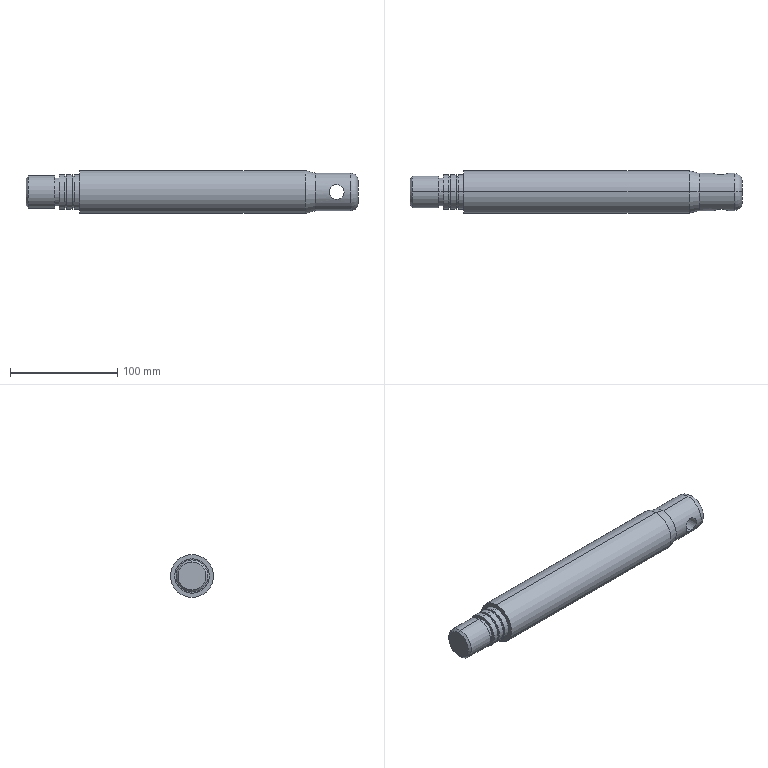Part | SolidWorks | features Chamfer 1, Fillet 1, ICE 1, Revolution 1 | 1 solid | 35 faces | box 310 x 40 x 40 mm | volume 342944 mm3 | cylinder 20 | plane 9 | cone 4 | torus 2 | commonest cylinder face diameters 32 x6 29 x4 14 x2 26 x2 30 x2 35 x2
STEP:
#1=CARTESIAN_POINT('',(310.,0.,-10.5));
#2=VERTEX_POINT('',#1);
#3=CARTESIAN_POINT('',(310.,0.,10.5));
#4=VERTEX_POINT('',#3);
#5=CARTESIAN_POINT('',(310.,0.,0.));
#6=DIRECTION('',(1.,0.,0.));
#7=DIRECTION('',(0.,0.,1.));
#8=AXIS2_PLACEMENT_3D('',#5,#6,#7);
#9=CIRCLE('',#8,10.5);
#10=EDGE_CURVE('',#2,#4,#9,.T.);
#11=ORIENTED_EDGE('',*,*,#10,.F.);
#12=CARTESIAN_POINT('',(303.,0.,-17.5));
#13=VERTEX_POINT('',#12);
#14=CARTESIAN_POINT('',(303.,0.,-10.5));
#15=DIRECTION('',(0.,1.,0.));
#16=DIRECTION('',(0.,0.,1.));
#17=AXIS2_PLACEMENT_3D('',#14,#15,#16);
#18=CIRCLE('',#17,7.);
#19=EDGE_CURVE('',#2,#13,#18,.T.);
#20=ORIENTED_EDGE('',*,*,#19,.T.);
#21=CARTESIAN_POINT('',(303.,0.,17.5));
#22=VERTEX_POINT('',#21);
#23=CARTESIAN_POINT('',(303.,0.,0.));
#24=DIRECTION('',(-1.,0.,0.));
#25=DIRECTION('',(0.,0.,1.));
#26=AXIS2_PLACEMENT_3D('',#23,#24,#25);
#27=CIRCLE('',#26,17.5);
#28=EDGE_CURVE('',#22,#13,#27,.T.);
#29=ORIENTED_EDGE('',*,*,#28,.F.);
#30=CARTESIAN_POINT('',(303.,0.,10.5));
#31=DIRECTION('',(0.,-1.,0.));
#32=DIRECTION('',(0.,0.,-1.));
#33=AXIS2_PLACEMENT_3D('',#30,#31,#32);
#34=CIRCLE('',#33,7.);
#35=EDGE_CURVE('',#4,#22,#34,.T.);
#36=ORIENTED_EDGE('',*,*,#35,.F.);
#37=EDGE_LOOP('',(#11,#20,#29,#36));
#38=FACE_OUTER_BOUND('',#37,.T.);
#39=CARTESIAN_POINT('',(303.,0.,0.));
#40=DIRECTION('',(-1.,0.,0.));
#41=DIRECTION('',(0.,0.,1.));
#42=AXIS2_PLACEMENT_3D('',#39,#40,#41);
#43=TOROIDAL_SURFACE('',#42,10.5,7.);
#44=ADVANCED_FACE('',(#38),#43,.T.);
#45=CARTESIAN_POINT('',(0.,0.,13.));
#46=VERTEX_POINT('',#45);
#47=CARTESIAN_POINT('',(0.,0.,-13.));
#48=VERTEX_POINT('',#47);
#49=CARTESIAN_POINT('',(0.,0.,0.));
#50=DIRECTION('',(-1.,0.,0.));
#51=DIRECTION('',(0.,0.,-1.));
#52=AXIS2_PLACEMENT_3D('',#49,#50,#51);
#53=CIRCLE('',#52,13.);
#54=EDGE_CURVE('',#46,#48,#53,.T.);
#55=ORIENTED_EDGE('',*,*,#54,.F.);
#56=CARTESIAN_POINT('',(2.,0.,15.));
#57=VERTEX_POINT('',#56);
#58=CARTESIAN_POINT('',(0.,0.,13.));
#59=DIRECTION('',(0.7071,0.,0.7071));
#60=VECTOR('',#59,1000.);
#61=LINE('',#58,#60);
#62=EDGE_CURVE('',#46,#57,#61,.T.);
#63=ORIENTED_EDGE('',*,*,#62,.T.);
#64=CARTESIAN_POINT('',(2.,0.,-15.));
#65=VERTEX_POINT('',#64);
#66=CARTESIAN_POINT('',(2.,0.,0.));
#67=DIRECTION('',(1.,0.,0.));
#68=DIRECTION('',(0.,0.,-1.));
#69=AXIS2_PLACEMENT_3D('',#66,#67,#68);
#70=CIRCLE('',#69,15.);
#71=EDGE_CURVE('',#65,#57,#70,.T.);
#72=ORIENTED_EDGE('',*,*,#71,.F.);
#73=CARTESIAN_POINT('',(0.,0.,-13.));
#74=DIRECTION('',(0.7071,0.,-0.7071));
#75=VECTOR('',#74,1000.);
#76=LINE('',#73,#75);
#77=EDGE_CURVE('',#48,#65,#76,.T.);
#78=ORIENTED_EDGE('',*,*,#77,.F.);
#79=EDGE_LOOP('',(#55,#63,#72,#78));
#80=FACE_OUTER_BOUND('',#79,.T.);
#81=CARTESIAN_POINT('',(0.,0.,0.));
#82=DIRECTION('',(1.,0.,0.));
#83=DIRECTION('',(0.,0.,-1.));
#84=AXIS2_PLACEMENT_3D('',#81,#82,#83);
#85=CONICAL_SURFACE('',#84,13.,0.7854);
#86=ADVANCED_FACE('',(#80),#85,.T.);
#87=CARTESIAN_POINT('',(290.,-16.039,-7.));
#88=VERTEX_POINT('',#87);
#89=CARTESIAN_POINT('',(290.,-16.039,7.));
#90=VERTEX_POINT('',#89);
#91=CARTESIAN_POINT('',(290.,-16.039,-7.));
#92=CARTESIAN_POINT('',(289.77,-16.039,-7.));
#93=CARTESIAN_POINT('',(289.54,-16.044,-6.989));
#94=CARTESIAN_POINT('',(289.079,-16.064,-6.943));
#95=CARTESIAN_POINT('',(288.847,-16.079,-6.908));
#96=CARTESIAN_POINT('',(288.167,-16.137,-6.771));
#97=CARTESIAN_POINT('',(287.729,-16.194,-6.637));
#98=CARTESIAN_POINT('',(287.095,-16.299,-6.373));
#99=CARTESIAN_POINT('',(286.886,-16.337,-6.273));
#100=CARTESIAN_POINT('',(286.483,-16.419,-6.057));
#101=CARTESIAN_POINT('',(286.288,-16.462,-5.939));
#102=CARTESIAN_POINT('',(285.724,-16.595,-5.561));
#103=CARTESIAN_POINT('',(285.373,-16.69,-5.272));
#104=CARTESIAN_POINT('',(284.728,-16.881,-4.627));
#105=CARTESIAN_POINT('',(284.441,-16.973,-4.278));
#106=CARTESIAN_POINT('',(284.062,-17.102,-3.714));
#107=CARTESIAN_POINT('',(283.945,-17.144,-3.519));
#108=CARTESIAN_POINT('',(283.728,-17.222,-3.116));
#109=CARTESIAN_POINT('',(283.628,-17.258,-2.907));
#110=CARTESIAN_POINT('',(283.363,-17.357,-2.273));
#111=CARTESIAN_POINT('',(283.229,-17.409,-1.836));
#112=CARTESIAN_POINT('',(283.047,-17.481,-0.9335));
#113=CARTESIAN_POINT('',(283.,-17.5,-0.4644));
#114=CARTESIAN_POINT('',(283.,-17.5,0.4581));
#115=CARTESIAN_POINT('',(283.045,-17.482,0.9167));
#116=CARTESIAN_POINT('',(283.227,-17.41,1.829));
#117=CARTESIAN_POINT('',(283.363,-17.357,2.27));
#118=CARTESIAN_POINT('',(283.626,-17.259,2.903));
#119=CARTESIAN_POINT('',(283.724,-17.223,3.109));
#120=CARTESIAN_POINT('',(283.941,-17.145,3.513));
#121=CARTESIAN_POINT('',(284.06,-17.103,3.711));
#122=CARTESIAN_POINT('',(284.44,-16.974,4.278));
#123=CARTESIAN_POINT('',(284.727,-16.881,4.627));
#124=CARTESIAN_POINT('',(285.209,-16.739,5.108));
#125=CARTESIAN_POINT('',(285.378,-16.691,5.262));
#126=CARTESIAN_POINT('',(285.73,-16.597,5.551));
#127=CARTESIAN_POINT('',(285.912,-16.551,5.687));
#128=CARTESIAN_POINT('',(286.475,-16.418,6.064));
#129=CARTESIAN_POINT('',(286.874,-16.335,6.28));
#130=CARTESIAN_POINT('',(287.725,-16.194,6.636));
#131=CARTESIAN_POINT('',(288.165,-16.137,6.771));
#132=CARTESIAN_POINT('',(288.841,-16.079,6.907));
#133=CARTESIAN_POINT('',(289.069,-16.064,6.942));
#134=CARTESIAN_POINT('',(289.532,-16.044,6.988));
#135=CARTESIAN_POINT('',(289.766,-16.039,7.));
#136=CARTESIAN_POINT('',(290.,-16.039,7.));
#137=B_SPLINE_CURVE_WITH_KNOTS('',3,(#91,#92,#93,#94,#95,#96,#97,#98,#99,#100,#101,#102,#103,#104,#105,#106,#107,#108,#109,#110,#111,#112,#113,#114,#115,#116,#117,#118,#119,#120,#121,#122,#123,#124,#125,#126,#127,#128,#129,#130,#131,#132,#133,#134,#135,#136),.UNSPECIFIED.,.F.,.F.,(4,2,2,2,2,2,2,2,2,2,2,2,2,2,2,2,2,2,2,2,2,2,4),(0.02212,0.02281,0.0235,0.02488,0.02557,0.02626,0.02764,0.02902,0.02971,0.0304,0.03179,0.03317,0.03455,0.03593,0.03662,0.03731,0.03869,0.03938,0.04007,0.04145,0.04283,0.04353,0.04422),.UNSPECIFIED.);
#138=EDGE_CURVE('',#88,#90,#137,.T.);
#139=ORIENTED_EDGE('',*,*,#138,.F.);
#140=CARTESIAN_POINT('',(290.,16.039,-7.));
#141=VERTEX_POINT('',#140);
#142=CARTESIAN_POINT('',(290.,-20.,-7.));
#143=DIRECTION('',(0.,1.,0.));
#144=VECTOR('',#143,1000.);
#145=LINE('',#142,#144);
#146=EDGE_CURVE('',#88,#141,#145,.T.);
#147=ORIENTED_EDGE('',*,*,#146,.T.);
#148=CARTESIAN_POINT('',(290.,16.039,7.));
#149=VERTEX_POINT('',#148);
#150=CARTESIAN_POINT('',(290.,16.039,7.));
#151=CARTESIAN_POINT('',(289.532,16.039,7.));
#152=CARTESIAN_POINT('',(289.073,16.059,6.954));
#153=CARTESIAN_POINT('',(288.397,16.117,6.818));
#154=CARTESIAN_POINT('',(288.174,16.141,6.762));
#155=CARTESIAN_POINT('',(287.732,16.197,6.626));
#156=CARTESIAN_POINT('',(287.514,16.229,6.548));
#157=CARTESIAN_POINT('',(286.88,16.334,6.283));
#158=CARTESIAN_POINT('',(286.48,16.417,6.068));
#159=CARTESIAN_POINT('',(285.912,16.551,5.687));
#160=CARTESIAN_POINT('',(285.728,16.597,5.55));
#161=CARTESIAN_POINT('',(285.377,16.691,5.261));
#162=CARTESIAN_POINT('',(285.21,16.738,5.109));
#163=CARTESIAN_POINT('',(284.731,16.88,4.63));
#164=CARTESIAN_POINT('',(284.441,16.973,4.279));
#165=CARTESIAN_POINT('',(283.931,17.147,3.518));
#166=CARTESIAN_POINT('',(283.716,17.225,3.118));
#167=CARTESIAN_POINT('',(283.453,17.324,2.487));
#168=CARTESIAN_POINT('',(283.375,17.353,2.271));
#169=CARTESIAN_POINT('',(283.24,17.405,1.83));
#170=CARTESIAN_POINT('',(283.182,17.428,1.603));
#171=CARTESIAN_POINT('',(283.046,17.482,0.9238));
#172=CARTESIAN_POINT('',(283.,17.5,0.466));
#173=CARTESIAN_POINT('',(283.,17.5,-0.2276));
#174=CARTESIAN_POINT('',(283.011,17.495,-0.4612));
#175=CARTESIAN_POINT('',(283.057,17.477,-0.9248));
#176=CARTESIAN_POINT('',(283.092,17.463,-1.153));
#177=CARTESIAN_POINT('',(283.228,17.41,-1.83));
#178=CARTESIAN_POINT('',(283.362,17.358,-2.27));
#179=CARTESIAN_POINT('',(283.719,17.224,-3.124));
#180=CARTESIAN_POINT('',(283.935,17.146,-3.525));
#181=CARTESIAN_POINT('',(284.441,16.973,-4.279));
#182=CARTESIAN_POINT('',(284.734,16.878,-4.635));
#183=CARTESIAN_POINT('',(285.376,16.689,-5.275));
#184=CARTESIAN_POINT('',(285.725,16.595,-5.561));
#185=CARTESIAN_POINT('',(286.292,16.461,-5.941));
#186=CARTESIAN_POINT('',(286.489,16.418,-6.06));
#187=CARTESIAN_POINT('',(286.892,16.336,-6.276));
#188=CARTESIAN_POINT('',(287.098,16.298,-6.374));
#189=CARTESIAN_POINT('',(287.728,16.194,-6.637));
#190=CARTESIAN_POINT('',(288.166,16.137,-6.771));
#191=CARTESIAN_POINT('',(288.849,16.079,-6.909));
#192=CARTESIAN_POINT('',(289.08,16.064,-6.943));
#193=CARTESIAN_POINT('',(289.54,16.044,-6.989));
#194=CARTESIAN_POINT('',(289.77,16.039,-7.));
#195=CARTESIAN_POINT('',(290.,16.039,-7.));
#196=B_SPLINE_CURVE_WITH_KNOTS('',3,(#150,#151,#152,#153,#154,#155,#156,#157,#158,#159,#160,#161,#162,#163,#164,#165,#166,#167,#168,#169,#170,#171,#172,#173,#174,#175,#176,#177,#178,#179,#180,#181,#182,#183,#184,#185,#186,#187,#188,#189,#190,#191,#192,#193,#194,#195),.UNSPECIFIED.,.F.,.F.,(4,2,2,2,2,2,2,2,2,2,2,2,2,2,2,2,2,2,2,2,2,2,4),(0.,0.001382,0.002074,0.002765,0.004147,0.004838,0.00553,0.006912,0.008294,0.008985,0.009677,0.01106,0.01175,0.01244,0.01382,0.01521,0.01659,0.01797,0.01866,0.01935,0.02074,0.02143,0.02212),.UNSPECIFIED.);
#197=EDGE_CURVE('',#149,#141,#196,.T.);
#198=ORIENTED_EDGE('',*,*,#197,.F.);
#199=CARTESIAN_POINT('',(290.,-20.,7.));
#200=DIRECTION('',(0.,1.,0.));
#201=VECTOR('',#200,1000.);
#202=LINE('',#199,#201);
#203=EDGE_CURVE('',#90,#149,#202,.T.);
#204=ORIENTED_EDGE('',*,*,#203,.F.);
#205=EDGE_LOOP('',(#139,#147,#198,#204));
#206=FACE_OUTER_BOUND('',#205,.T.);
#207=CARTESIAN_POINT('',(290.,-20.,0.));
#208=DIRECTION('',(0.,1.,0.));
#209=DIRECTION('',(0.,0.,1.));
#210=AXIS2_PLACEMENT_3D('',#207,#208,#209);
#211=CYLINDRICAL_SURFACE('',#210,7.);
#212=ADVANCED_FACE('',(#206),#211,.F.);
#213=ORIENTED_EDGE('',*,*,#197,.T.);
#214=CARTESIAN_POINT('',(290.,16.039,-7.));
#215=CARTESIAN_POINT('',(290.23,16.039,-7.));
#216=CARTESIAN_POINT('',(290.46,16.044,-6.989));
#217=CARTESIAN_POINT('',(290.921,16.064,-6.943));
#218=CARTESIAN_POINT('',(291.153,16.079,-6.908));
#219=CARTESIAN_POINT('',(291.833,16.137,-6.771));
#220=CARTESIAN_POINT('',(292.271,16.194,-6.637));
#221=CARTESIAN_POINT('',(292.905,16.299,-6.373));
#222=CARTESIAN_POINT('',(293.114,16.337,-6.273));
#223=CARTESIAN_POINT('',(293.517,16.419,-6.057));
#224=CARTESIAN_POINT('',(293.712,16.462,-5.939));
#225=CARTESIAN_POINT('',(294.276,16.595,-5.561));
#226=CARTESIAN_POINT('',(294.627,16.69,-5.272));
#227=CARTESIAN_POINT('',(295.272,16.881,-4.627));
#228=CARTESIAN_POINT('',(295.559,16.973,-4.278));
#229=CARTESIAN_POINT('',(295.938,17.102,-3.714));
#230=CARTESIAN_POINT('',(296.055,17.144,-3.519));
#231=CARTESIAN_POINT('',(296.272,17.222,-3.116));
#232=CARTESIAN_POINT('',(296.372,17.258,-2.907));
#233=CARTESIAN_POINT('',(296.637,17.357,-2.273));
#234=CARTESIAN_POINT('',(296.771,17.409,-1.836));
#235=CARTESIAN_POINT('',(296.953,17.481,-0.9335));
#236=CARTESIAN_POINT('',(297.,17.5,-0.4644));
#237=CARTESIAN_POINT('',(297.,17.5,0.4581));
#238=CARTESIAN_POINT('',(296.955,17.482,0.9167));
#239=CARTESIAN_POINT('',(296.773,17.41,1.829));
#240=CARTESIAN_POINT('',(296.637,17.357,2.27));
#241=CARTESIAN_POINT('',(296.374,17.259,2.903));
#242=CARTESIAN_POINT('',(296.276,17.223,3.109));
#243=CARTESIAN_POINT('',(296.059,17.145,3.513));
#244=CARTESIAN_POINT('',(295.94,17.103,3.711));
#245=CARTESIAN_POINT('',(295.56,16.974,4.278));
#246=CARTESIAN_POINT('',(295.273,16.881,4.627));
#247=CARTESIAN_POINT('',(294.791,16.739,5.108));
#248=CARTESIAN_POINT('',(294.622,16.691,5.262));
#249=CARTESIAN_POINT('',(294.27,16.597,5.551));
#250=CARTESIAN_POINT('',(294.088,16.551,5.687));
#251=CARTESIAN_POINT('',(293.525,16.418,6.064));
#252=CARTESIAN_POINT('',(293.126,16.335,6.28));
#253=CARTESIAN_POINT('',(292.275,16.194,6.636));
#254=CARTESIAN_POINT('',(291.835,16.137,6.771));
#255=CARTESIAN_POINT('',(291.159,16.079,6.907));
#256=CARTESIAN_POINT('',(290.931,16.064,6.942));
#257=CARTESIAN_POINT('',(290.468,16.044,6.988));
#258=CARTESIAN_POINT('',(290.234,16.039,7.));
#259=CARTESIAN_POINT('',(290.,16.039,7.));
#260=B_SPLINE_CURVE_WITH_KNOTS('',3,(#214,#215,#216,#217,#218,#219,#220,#221,#222,#223,#224,#225,#226,#227,#228,#229,#230,#231,#232,#233,#234,#235,#236,#237,#238,#239,#240,#241,#242,#243,#244,#245,#246,#247,#248,#249,#250,#251,#252,#253,#254,#255,#256,#257,#258,#259),.UNSPECIFIED.,.F.,.F.,(4,2,2,2,2,2,2,2,2,2,2,2,2,2,2,2,2,2,2,2,2,2,4),(0.02212,0.02281,0.0235,0.02488,0.02557,0.02626,0.02764,0.02902,0.02971,0.0304,0.03179,0.03317,0.03455,0.03593,0.03662,0.03731,0.03869,0.03938,0.04007,0.04145,0.04283,0.04353,0.04422),.UNSPECIFIED.);
#261=EDGE_CURVE('',#141,#149,#260,.T.);
#262=ORIENTED_EDGE('',*,*,#261,.T.);
#263=EDGE_LOOP('',(#213,#262));
#264=FACE_BOUND('',#263,.T.);
#265=ORIENTED_EDGE('',*,*,#28,.T.);
#266=CARTESIAN_POINT('',(270.,0.,-17.5));
#267=VERTEX_POINT('',#266);
#268=CARTESIAN_POINT('',(0.,0.,-17.5));
#269=DIRECTION('',(-1.,0.,0.));
#270=VECTOR('',#269,1000.);
#271=LINE('',#268,#270);
#272=EDGE_CURVE('',#13,#267,#271,.T.);
#273=ORIENTED_EDGE('',*,*,#272,.T.);
#274=CARTESIAN_POINT('',(270.,0.,17.5));
#275=VERTEX_POINT('',#274);
#276=CARTESIAN_POINT('',(270.,0.,0.));
#277=DIRECTION('',(-1.,0.,0.));
#278=DIRECTION('',(0.,0.,1.));
#279=AXIS2_PLACEMENT_3D('',#276,#277,#278);
#280=CIRCLE('',#279,17.5);
#281=EDGE_CURVE('',#275,#267,#280,.T.);
#282=ORIENTED_EDGE('',*,*,#281,.F.);
#283=CARTESIAN_POINT('',(0.,0.,17.5));
#284=DIRECTION('',(-1.,0.,0.));
#285=VECTOR('',#284,1000.);
#286=LINE('',#283,#285);
#287=EDGE_CURVE('',#22,#275,#286,.T.);
#288=ORIENTED_EDGE('',*,*,#287,.F.);
#289=EDGE_LOOP('',(#265,#273,#282,#288));
#290=FACE_OUTER_BOUND('',#289,.T.);
#291=CARTESIAN_POINT('',(0.,0.,0.));
#292=DIRECTION('',(-1.,0.,0.));
#293=DIRECTION('',(0.,0.,1.));
#294=AXIS2_PLACEMENT_3D('',#291,#292,#293);
#295=CYLINDRICAL_SURFACE('',#294,17.5);
#296=ADVANCED_FACE('',(#264,#290),#295,.T.);
#297=ORIENTED_EDGE('',*,*,#281,.T.);
#298=CARTESIAN_POINT('',(260.67,0.,-20.));
#299=VERTEX_POINT('',#298);
#300=CARTESIAN_POINT('',(270.,0.,-17.5));
#301=DIRECTION('',(-0.9659,0.,-0.2588));
#302=VECTOR('',#301,1000.);
#303=LINE('',#300,#302);
#304=EDGE_CURVE('',#267,#299,#303,.T.);
#305=ORIENTED_EDGE('',*,*,#304,.T.);
#306=CARTESIAN_POINT('',(260.67,0.,20.));
#307=VERTEX_POINT('',#306);
#308=CARTESIAN_POINT('',(260.67,0.,0.));
#309=DIRECTION('',(-1.,0.,0.));
#310=DIRECTION('',(0.,0.,1.));
#311=AXIS2_PLACEMENT_3D('',#308,#309,#310);
#312=CIRCLE('',#311,20.);
#313=EDGE_CURVE('',#307,#299,#312,.T.);
#314=ORIENTED_EDGE('',*,*,#313,.F.);
#315=CARTESIAN_POINT('',(270.,0.,17.5));
#316=DIRECTION('',(-0.9659,0.,0.2588));
#317=VECTOR('',#316,1000.);
#318=LINE('',#315,#317);
#319=EDGE_CURVE('',#275,#307,#318,.T.);
#320=ORIENTED_EDGE('',*,*,#319,.F.);
#321=EDGE_LOOP('',(#297,#305,#314,#320));
#322=FACE_OUTER_BOUND('',#321,.T.);
#323=CARTESIAN_POINT('',(270.,0.,0.));
#324=DIRECTION('',(-1.,0.,0.));
#325=DIRECTION('',(0.,0.,1.));
#326=AXIS2_PLACEMENT_3D('',#323,#324,#325);
#327=CONICAL_SURFACE('',#326,17.5,0.2618);
#328=ADVANCED_FACE('',(#322),#327,.T.);
#329=ORIENTED_EDGE('',*,*,#313,.T.);
#330=CARTESIAN_POINT('',(50.,0.,-20.));
#331=VERTEX_POINT('',#330);
#332=CARTESIAN_POINT('',(0.,0.,-20.));
#333=DIRECTION('',(-1.,0.,0.));
#334=VECTOR('',#333,1000.);
#335=LINE('',#332,#334);
#336=EDGE_CURVE('',#299,#331,#335,.T.);
#337=ORIENTED_EDGE('',*,*,#336,.T.);
#338=CARTESIAN_POINT('',(50.,0.,20.));
#339=VERTEX_POINT('',#338);
#340=CARTESIAN_POINT('',(50.,0.,0.));
#341=DIRECTION('',(-1.,0.,0.));
#342=DIRECTION('',(0.,0.,1.));
#343=AXIS2_PLACEMENT_3D('',#340,#341,#342);
#344=CIRCLE('',#343,20.);
#345=EDGE_CURVE('',#339,#331,#344,.T.);
#346=ORIENTED_EDGE('',*,*,#345,.F.);
#347=CARTESIAN_POINT('',(0.,0.,20.));
#348=DIRECTION('',(-1.,0.,0.));
#349=VECTOR('',#348,1000.);
#350=LINE('',#347,#349);
#351=EDGE_CURVE('',#307,#339,#350,.T.);
#352=ORIENTED_EDGE('',*,*,#351,.F.);
#353=EDGE_LOOP('',(#329,#337,#346,#352));
#354=FACE_OUTER_BOUND('',#353,.T.);
#355=CARTESIAN_POINT('',(0.,0.,0.));
#356=DIRECTION('',(-1.,0.,0.));
#357=DIRECTION('',(0.,0.,1.));
#358=AXIS2_PLACEMENT_3D('',#355,#356,#357);
#359=CYLINDRICAL_SURFACE('',#358,20.);
#360=ADVANCED_FACE('',(#354),#359,.T.);
#361=CARTESIAN_POINT('',(50.,0.,16.));
#362=VERTEX_POINT('',#361);
#363=CARTESIAN_POINT('',(50.,0.,-16.));
#364=VERTEX_POINT('',#363);
#365=CARTESIAN_POINT('',(50.,0.,0.));
#366=DIRECTION('',(-1.,0.,0.));
#367=DIRECTION('',(0.,0.,1.));
#368=AXIS2_PLACEMENT_3D('',#365,#366,#367);
#369=CIRCLE('',#368,16.);
#370=EDGE_CURVE('',#362,#364,#369,.T.);
#371=ORIENTED_EDGE('',*,*,#370,.T.);
#372=CARTESIAN_POINT('',(45.,0.,-16.));
#373=VERTEX_POINT('',#372);
#374=CARTESIAN_POINT('',(0.,0.,-16.));
#375=DIRECTION('',(-1.,0.,0.));
#376=VECTOR('',#375,1000.);
#377=LINE('',#374,#376);
#378=EDGE_CURVE('',#364,#373,#377,.T.);
#379=ORIENTED_EDGE('',*,*,#378,.T.);
#380=CARTESIAN_POINT('',(45.,0.,16.));
#381=VERTEX_POINT('',#380);
#382=CARTESIAN_POINT('',(45.,0.,0.));
#383=DIRECTION('',(-1.,0.,0.));
#384=DIRECTION('',(0.,0.,1.));
#385=AXIS2_PLACEMENT_3D('',#382,#383,#384);
#386=CIRCLE('',#385,16.);
#387=EDGE_CURVE('',#381,#373,#386,.T.);
#388=ORIENTED_EDGE('',*,*,#387,.F.);
#389=CARTESIAN_POINT('',(0.,0.,16.));
#390=DIRECTION('',(-1.,0.,0.));
#391=VECTOR('',#390,1000.);
#392=LINE('',#389,#391);
#393=EDGE_CURVE('',#362,#381,#392,.T.);
#394=ORIENTED_EDGE('',*,*,#393,.F.);
#395=EDGE_LOOP('',(#371,#379,#388,#394));
#396=FACE_OUTER_BOUND('',#395,.T.);
#397=CARTESIAN_POINT('',(0.,0.,0.));
#398=DIRECTION('',(-1.,0.,0.));
#399=DIRECTION('',(0.,0.,1.));
#400=AXIS2_PLACEMENT_3D('',#397,#398,#399);
#401=CYLINDRICAL_SURFACE('',#400,16.);
#402=ADVANCED_FACE('',(#396),#401,.T.);
#403=CARTESIAN_POINT('',(45.,0.,14.5));
#404=VERTEX_POINT('',#403);
#405=CARTESIAN_POINT('',(45.,0.,-14.5));
#406=VERTEX_POINT('',#405);
#407=CARTESIAN_POINT('',(45.,0.,0.));
#408=DIRECTION('',(-1.,0.,0.));
#409=DIRECTION('',(0.,0.,1.));
#410=AXIS2_PLACEMENT_3D('',#407,#408,#409);
#411=CIRCLE('',#410,14.5);
#412=EDGE_CURVE('',#404,#406,#411,.T.);
#413=ORIENTED_EDGE('',*,*,#412,.T.);
#414=CARTESIAN_POINT('',(43.,0.,-14.5));
#415=VERTEX_POINT('',#414);
#416=CARTESIAN_POINT('',(0.,0.,-14.5));
#417=DIRECTION('',(-1.,0.,0.));
#418=VECTOR('',#417,1000.);
#419=LINE('',#416,#418);
#420=EDGE_CURVE('',#406,#415,#419,.T.);
#421=ORIENTED_EDGE('',*,*,#420,.T.);
#422=CARTESIAN_POINT('',(43.,0.,14.5));
#423=VERTEX_POINT('',#422);
#424=CARTESIAN_POINT('',(43.,0.,0.));
#425=DIRECTION('',(-1.,0.,0.));
#426=DIRECTION('',(0.,0.,1.));
#427=AXIS2_PLACEMENT_3D('',#424,#425,#426);
#428=CIRCLE('',#427,14.5);
#429=EDGE_CURVE('',#423,#415,#428,.T.);
#430=ORIENTED_EDGE('',*,*,#429,.F.);
#431=CARTESIAN_POINT('',(0.,0.,14.5));
#432=DIRECTION('',(-1.,0.,0.));
#433=VECTOR('',#432,1000.);
#434=LINE('',#431,#433);
#435=EDGE_CURVE('',#404,#423,#434,.T.);
#436=ORIENTED_EDGE('',*,*,#435,.F.);
#437=EDGE_LOOP('',(#413,#421,#430,#436));
#438=FACE_OUTER_BOUND('',#437,.T.);
#439=CARTESIAN_POINT('',(0.,0.,0.));
#440=DIRECTION('',(-1.,0.,0.));
#441=DIRECTION('',(0.,0.,1.));
#442=AXIS2_PLACEMENT_3D('',#439,#440,#441);
#443=CYLINDRICAL_SURFACE('',#442,14.5);
#444=ADVANCED_FACE('',(#438),#443,.T.);
#445=CARTESIAN_POINT('',(43.,0.,16.));
#446=VERTEX_POINT('',#445);
#447=CARTESIAN_POINT('',(43.,0.,-16.));
#448=VERTEX_POINT('',#447);
#449=CARTESIAN_POINT('',(43.,0.,0.));
#450=DIRECTION('',(-1.,0.,0.));
#451=DIRECTION('',(0.,0.,1.));
#452=AXIS2_PLACEMENT_3D('',#449,#450,#451);
#453=CIRCLE('',#452,16.);
#454=EDGE_CURVE('',#446,#448,#453,.T.);
#455=ORIENTED_EDGE('',*,*,#454,.T.);
#456=CARTESIAN_POINT('',(38.,0.,-16.));
#457=VERTEX_POINT('',#456);
#458=CARTESIAN_POINT('',(0.,0.,-16.));
#459=DIRECTION('',(-1.,0.,0.));
#460=VECTOR('',#459,1000.);
#461=LINE('',#458,#460);
#462=EDGE_CURVE('',#448,#457,#461,.T.);
#463=ORIENTED_EDGE('',*,*,#462,.T.);
#464=CARTESIAN_POINT('',(38.,0.,16.));
#465=VERTEX_POINT('',#464);
#466=CARTESIAN_POINT('',(38.,0.,0.));
#467=DIRECTION('',(-1.,0.,0.));
#468=DIRECTION('',(0.,0.,1.));
#469=AXIS2_PLACEMENT_3D('',#466,#467,#468);
#470=CIRCLE('',#469,16.);
#471=EDGE_CURVE('',#465,#457,#470,.T.);
#472=ORIENTED_EDGE('',*,*,#471,.F.);
#473=CARTESIAN_POINT('',(0.,0.,16.));
#474=DIRECTION('',(-1.,0.,0.));
#475=VECTOR('',#474,1000.);
#476=LINE('',#473,#475);
#477=EDGE_CURVE('',#446,#465,#476,.T.);
#478=ORIENTED_EDGE('',*,*,#477,.F.);
#479=EDGE_LOOP('',(#455,#463,#472,#478));
#480=FACE_OUTER_BOUND('',#479,.T.);
#481=CARTESIAN_POINT('',(0.,0.,0.));
#482=DIRECTION('',(-1.,0.,0.));
#483=DIRECTION('',(0.,0.,1.));
#484=AXIS2_PLACEMENT_3D('',#481,#482,#483);
#485=CYLINDRICAL_SURFACE('',#484,16.);
#486=ADVANCED_FACE('',(#480),#485,.T.);
#487=CARTESIAN_POINT('',(38.,0.,14.5));
#488=VERTEX_POINT('',#487);
#489=CARTESIAN_POINT('',(38.,0.,-14.5));
#490=VERTEX_POINT('',#489);
#491=CARTESIAN_POINT('',(38.,0.,0.));
#492=DIRECTION('',(-1.,0.,0.));
#493=DIRECTION('',(0.,0.,1.));
#494=AXIS2_PLACEMENT_3D('',#491,#492,#493);
#495=CIRCLE('',#494,14.5);
#496=EDGE_CURVE('',#488,#490,#495,.T.);
#497=ORIENTED_EDGE('',*,*,#496,.T.);
#498=CARTESIAN_POINT('',(36.,0.,-14.5));
#499=VERTEX_POINT('',#498);
#500=CARTESIAN_POINT('',(0.,0.,-14.5));
#501=DIRECTION('',(-1.,0.,0.));
#502=VECTOR('',#501,1000.);
#503=LINE('',#500,#502);
#504=EDGE_CURVE('',#490,#499,#503,.T.);
#505=ORIENTED_EDGE('',*,*,#504,.T.);
#506=CARTESIAN_POINT('',(36.,0.,14.5));
#507=VERTEX_POINT('',#506);
#508=CARTESIAN_POINT('',(36.,0.,0.));
#509=DIRECTION('',(-1.,0.,0.));
#510=DIRECTION('',(0.,0.,1.));
#511=AXIS2_PLACEMENT_3D('',#508,#509,#510);
#512=CIRCLE('',#511,14.5);
#513=EDGE_CURVE('',#507,#499,#512,.T.);
#514=ORIENTED_EDGE('',*,*,#513,.F.);
#515=CARTESIAN_POINT('',(0.,0.,14.5));
#516=DIRECTION('',(-1.,0.,0.));
#517=VECTOR('',#516,1000.);
#518=LINE('',#515,#517);
#519=EDGE_CURVE('',#488,#507,#518,.T.);
#520=ORIENTED_EDGE('',*,*,#519,.F.);
#521=EDGE_LOOP('',(#497,#505,#514,#520));
#522=FACE_OUTER_BOUND('',#521,.T.);
#523=CARTESIAN_POINT('',(0.,0.,0.));
#524=DIRECTION('',(-1.,0.,0.));
#525=DIRECTION('',(0.,0.,1.));
#526=AXIS2_PLACEMENT_3D('',#523,#524,#525);
#527=CYLINDRICAL_SURFACE('',#526,14.5);
#528=ADVANCED_FACE('',(#522),#527,.T.);
#529=CARTESIAN_POINT('',(36.,0.,16.));
#530=VERTEX_POINT('',#529);
#531=CARTESIAN_POINT('',(36.,0.,-16.));
#532=VERTEX_POINT('',#531);
#533=CARTESIAN_POINT('',(36.,0.,0.));
#534=DIRECTION('',(-1.,0.,0.));
#535=DIRECTION('',(0.,0.,1.));
#536=AXIS2_PLACEMENT_3D('',#533,#534,#535);
#537=CIRCLE('',#536,16.);
#538=EDGE_CURVE('',#530,#532,#537,.T.);
#539=ORIENTED_EDGE('',*,*,#538,.T.);
#540=CARTESIAN_POINT('',(31.,0.,-16.));
#541=VERTEX_POINT('',#540);
#542=CARTESIAN_POINT('',(0.,0.,-16.));
#543=DIRECTION('',(-1.,0.,0.));
#544=VECTOR('',#543,1000.);
#545=LINE('',#542,#544);
#546=EDGE_CURVE('',#532,#541,#545,.T.);
#547=ORIENTED_EDGE('',*,*,#546,.T.);
#548=CARTESIAN_POINT('',(31.,0.,16.));
#549=VERTEX_POINT('',#548);
#550=CARTESIAN_POINT('',(31.,0.,0.));
#551=DIRECTION('',(-1.,0.,0.));
#552=DIRECTION('',(0.,0.,1.));
#553=AXIS2_PLACEMENT_3D('',#550,#551,#552);
#554=CIRCLE('',#553,16.);
#555=EDGE_CURVE('',#549,#541,#554,.T.);
#556=ORIENTED_EDGE('',*,*,#555,.F.);
#557=CARTESIAN_POINT('',(0.,0.,16.));
#558=DIRECTION('',(-1.,0.,0.));
#559=VECTOR('',#558,1000.);
#560=LINE('',#557,#559);
#561=EDGE_CURVE('',#530,#549,#560,.T.);
#562=ORIENTED_EDGE('',*,*,#561,.F.);
#563=EDGE_LOOP('',(#539,#547,#556,#562));
#564=FACE_OUTER_BOUND('',#563,.T.);
#565=CARTESIAN_POINT('',(0.,0.,0.));
#566=DIRECTION('',(-1.,0.,0.));
#567=DIRECTION('',(0.,0.,1.));
#568=AXIS2_PLACEMENT_3D('',#565,#566,#567);
#569=CYLINDRICAL_SURFACE('',#568,16.);
#570=ADVANCED_FACE('',(#564),#569,.T.);
#571=CARTESIAN_POINT('',(31.,0.,13.));
#572=VERTEX_POINT('',#571);
#573=CARTESIAN_POINT('',(31.,0.,-13.));
#574=VERTEX_POINT('',#573);
#575=CARTESIAN_POINT('',(31.,0.,0.));
#576=DIRECTION('',(-1.,0.,0.));
#577=DIRECTION('',(0.,0.,1.));
#578=AXIS2_PLACEMENT_3D('',#575,#576,#577);
#579=CIRCLE('',#578,13.);
#580=EDGE_CURVE('',#572,#574,#579,.T.);
#581=ORIENTED_EDGE('',*,*,#580,.T.);
#582=CARTESIAN_POINT('',(27.,0.,-13.));
#583=VERTEX_POINT('',#582);
#584=CARTESIAN_POINT('',(0.,0.,-13.));
#585=DIRECTION('',(-1.,0.,0.));
#586=VECTOR('',#585,1000.);
#587=LINE('',#584,#586);
#588=EDGE_CURVE('',#574,#583,#587,.T.);
#589=ORIENTED_EDGE('',*,*,#588,.T.);
#590=CARTESIAN_POINT('',(27.,0.,13.));
#591=VERTEX_POINT('',#590);
#592=CARTESIAN_POINT('',(27.,0.,0.));
#593=DIRECTION('',(-1.,0.,0.));
#594=DIRECTION('',(0.,0.,1.));
#595=AXIS2_PLACEMENT_3D('',#592,#593,#594);
#596=CIRCLE('',#595,13.);
#597=EDGE_CURVE('',#591,#583,#596,.T.);
#598=ORIENTED_EDGE('',*,*,#597,.F.);
#599=CARTESIAN_POINT('',(0.,0.,13.));
#600=DIRECTION('',(-1.,0.,0.));
#601=VECTOR('',#600,1000.);
#602=LINE('',#599,#601);
#603=EDGE_CURVE('',#572,#591,#602,.T.);
#604=ORIENTED_EDGE('',*,*,#603,.F.);
#605=EDGE_LOOP('',(#581,#589,#598,#604));
#606=FACE_OUTER_BOUND('',#605,.T.);
#607=CARTESIAN_POINT('',(0.,0.,0.));
#608=DIRECTION('',(-1.,0.,0.));
#609=DIRECTION('',(0.,0.,1.));
#610=AXIS2_PLACEMENT_3D('',#607,#608,#609);
#611=CYLINDRICAL_SURFACE('',#610,13.);
#612=ADVANCED_FACE('',(#606),#611,.T.);
#613=CARTESIAN_POINT('',(27.,0.,15.));
#614=VERTEX_POINT('',#613);
#615=CARTESIAN_POINT('',(27.,0.,-15.));
#616=VERTEX_POINT('',#615);
#617=CARTESIAN_POINT('',(27.,0.,0.));
#618=DIRECTION('',(-1.,0.,0.));
#619=DIRECTION('',(0.,0.,1.));
#620=AXIS2_PLACEMENT_3D('',#617,#618,#619);
#621=CIRCLE('',#620,15.);
#622=EDGE_CURVE('',#614,#616,#621,.T.);
#623=ORIENTED_EDGE('',*,*,#622,.T.);
#624=CARTESIAN_POINT('',(0.,0.,-15.));
#625=DIRECTION('',(-1.,0.,0.));
#626=VECTOR('',#625,1000.);
#627=LINE('',#624,#626);
#628=EDGE_CURVE('',#616,#65,#627,.T.);
#629=ORIENTED_EDGE('',*,*,#628,.T.);
#630=ORIENTED_EDGE('',*,*,#71,.T.);
#631=CARTESIAN_POINT('',(0.,0.,15.));
#632=DIRECTION('',(-1.,0.,0.));
#633=VECTOR('',#632,1000.);
#634=LINE('',#631,#633);
#635=EDGE_CURVE('',#614,#57,#634,.T.);
#636=ORIENTED_EDGE('',*,*,#635,.F.);
#637=EDGE_LOOP('',(#623,#629,#630,#636));
#638=FACE_OUTER_BOUND('',#637,.T.);
#639=CARTESIAN_POINT('',(0.,0.,0.));
#640=DIRECTION('',(-1.,0.,0.));
#641=DIRECTION('',(0.,0.,1.));
#642=AXIS2_PLACEMENT_3D('',#639,#640,#641);
#643=CYLINDRICAL_SURFACE('',#642,15.);
#644=ADVANCED_FACE('',(#638),#643,.T.);
#645=CARTESIAN_POINT('',(0.,0.,0.));
#646=DIRECTION('',(-1.,0.,0.));
#647=DIRECTION('',(0.,0.,-1.));
#648=AXIS2_PLACEMENT_3D('',#645,#646,#647);
#649=CIRCLE('',#648,13.);
#650=EDGE_CURVE('',#48,#46,#649,.T.);
#651=ORIENTED_EDGE('',*,*,#650,.T.);
#652=ORIENTED_EDGE('',*,*,#54,.T.);
#653=EDGE_LOOP('',(#651,#652));
#654=FACE_OUTER_BOUND('',#653,.T.);
#655=CARTESIAN_POINT('',(0.,0.,0.));
#656=DIRECTION('',(1.,0.,0.));
#657=DIRECTION('',(0.,0.,-1.));
#658=AXIS2_PLACEMENT_3D('',#655,#656,#657);
#659=PLANE('',#658);
#660=ADVANCED_FACE('',(#654),#659,.F.);
#661=ORIENTED_EDGE('',*,*,#628,.F.);
#662=CARTESIAN_POINT('',(27.,0.,0.));
#663=DIRECTION('',(-1.,0.,0.));
#664=DIRECTION('',(0.,0.,1.));
#665=AXIS2_PLACEMENT_3D('',#662,#663,#664);
#666=CIRCLE('',#665,15.);
#667=EDGE_CURVE('',#616,#614,#666,.T.);
#668=ORIENTED_EDGE('',*,*,#667,.T.);
#669=ORIENTED_EDGE('',*,*,#635,.T.);
#670=CARTESIAN_POINT('',(2.,0.,0.));
#671=DIRECTION('',(1.,0.,0.));
#672=DIRECTION('',(0.,0.,-1.));
#673=AXIS2_PLACEMENT_3D('',#670,#671,#672);
#674=CIRCLE('',#673,15.);
#675=EDGE_CURVE('',#57,#65,#674,.T.);
#676=ORIENTED_EDGE('',*,*,#675,.T.);
#677=EDGE_LOOP('',(#661,#668,#669,#676));
#678=FACE_OUTER_BOUND('',#677,.T.);
#679=CARTESIAN_POINT('',(0.,0.,0.));
#680=DIRECTION('',(-1.,0.,0.));
#681=DIRECTION('',(0.,0.,1.));
#682=AXIS2_PLACEMENT_3D('',#679,#680,#681);
#683=CYLINDRICAL_SURFACE('',#682,15.);
#684=ADVANCED_FACE('',(#678),#683,.T.);
#685=ORIENTED_EDGE('',*,*,#622,.F.);
#686=ORIENTED_EDGE('',*,*,#667,.F.);
#687=EDGE_LOOP('',(#685,#686));
#688=FACE_OUTER_BOUND('',#687,.T.);
#689=ORIENTED_EDGE('',*,*,#597,.T.);
#690=CARTESIAN_POINT('',(27.,0.,0.));
#691=DIRECTION('',(-1.,0.,0.));
#692=DIRECTION('',(0.,0.,1.));
#693=AXIS2_PLACEMENT_3D('',#690,#691,#692);
#694=CIRCLE('',#693,13.);
#695=EDGE_CURVE('',#583,#591,#694,.T.);
#696=ORIENTED_EDGE('',*,*,#695,.T.);
#697=EDGE_LOOP('',(#689,#696));
#698=FACE_BOUND('',#697,.T.);
#699=CARTESIAN_POINT('',(27.,15.,0.));
#700=DIRECTION('',(-1.,0.,0.));
#701=DIRECTION('',(0.,0.,1.));
#702=AXIS2_PLACEMENT_3D('',#699,#700,#701);
#703=PLANE('',#702);
#704=ADVANCED_FACE('',(#688,#698),#703,.F.);
#705=ORIENTED_EDGE('',*,*,#588,.F.);
#706=CARTESIAN_POINT('',(31.,0.,0.));
#707=DIRECTION('',(-1.,0.,0.));
#708=DIRECTION('',(0.,0.,1.));
#709=AXIS2_PLACEMENT_3D('',#706,#707,#708);
#710=CIRCLE('',#709,13.);
#711=EDGE_CURVE('',#574,#572,#710,.T.);
#712=ORIENTED_EDGE('',*,*,#711,.T.);
#713=ORIENTED_EDGE('',*,*,#603,.T.);
#714=ORIENTED_EDGE('',*,*,#695,.F.);
#715=EDGE_LOOP('',(#705,#712,#713,#714));
#716=FACE_OUTER_BOUND('',#715,.T.);
#717=CARTESIAN_POINT('',(0.,0.,0.));
#718=DIRECTION('',(-1.,0.,0.));
#719=DIRECTION('',(0.,0.,1.));
#720=AXIS2_PLACEMENT_3D('',#717,#718,#719);
#721=CYLINDRICAL_SURFACE('',#720,13.);
#722=ADVANCED_FACE('',(#716),#721,.T.);
#723=ORIENTED_EDGE('',*,*,#580,.F.);
#724=ORIENTED_EDGE('',*,*,#711,.F.);
#725=EDGE_LOOP('',(#723,#724));
#726=FACE_BOUND('',#725,.T.);
#727=ORIENTED_EDGE('',*,*,#555,.T.);
#728=CARTESIAN_POINT('',(31.,0.,0.));
#729=DIRECTION('',(-1.,0.,0.));
#730=DIRECTION('',(0.,0.,1.));
#731=AXIS2_PLACEMENT_3D('',#728,#729,#730);
#732=CIRCLE('',#731,16.);
#733=EDGE_CURVE('',#541,#549,#732,.T.);
#734=ORIENTED_EDGE('',*,*,#733,.T.);
#735=EDGE_LOOP('',(#727,#734));
#736=FACE_OUTER_BOUND('',#735,.T.);
#737=CARTESIAN_POINT('',(31.,13.,0.));
#738=DIRECTION('',(1.,0.,0.));
#739=DIRECTION('',(0.,0.,-1.));
#740=AXIS2_PLACEMENT_3D('',#737,#738,#739);
#741=PLANE('',#740);
#742=ADVANCED_FACE('',(#726,#736),#741,.F.);
#743=ORIENTED_EDGE('',*,*,#546,.F.);
#744=CARTESIAN_POINT('',(36.,0.,0.));
#745=DIRECTION('',(-1.,0.,0.));
#746=DIRECTION('',(0.,0.,1.));
#747=AXIS2_PLACEMENT_3D('',#744,#745,#746);
#748=CIRCLE('',#747,16.);
#749=EDGE_CURVE('',#532,#530,#748,.T.);
#750=ORIENTED_EDGE('',*,*,#749,.T.);
#751=ORIENTED_EDGE('',*,*,#561,.T.);
#752=ORIENTED_EDGE('',*,*,#733,.F.);
#753=EDGE_LOOP('',(#743,#750,#751,#752));
#754=FACE_OUTER_BOUND('',#753,.T.);
#755=CARTESIAN_POINT('',(0.,0.,0.));
#756=DIRECTION('',(-1.,0.,0.));
#757=DIRECTION('',(0.,0.,1.));
#758=AXIS2_PLACEMENT_3D('',#755,#756,#757);
#759=CYLINDRICAL_SURFACE('',#758,16.);
#760=ADVANCED_FACE('',(#754),#759,.T.);
#761=ORIENTED_EDGE('',*,*,#538,.F.);
#762=ORIENTED_EDGE('',*,*,#749,.F.);
#763=EDGE_LOOP('',(#761,#762));
#764=FACE_OUTER_BOUND('',#763,.T.);
#765=ORIENTED_EDGE('',*,*,#513,.T.);
#766=CARTESIAN_POINT('',(36.,0.,0.));
#767=DIRECTION('',(-1.,0.,0.));
#768=DIRECTION('',(0.,0.,1.));
#769=AXIS2_PLACEMENT_3D('',#766,#767,#768);
#770=CIRCLE('',#769,14.5);
#771=EDGE_CURVE('',#499,#507,#770,.T.);
#772=ORIENTED_EDGE('',*,*,#771,.T.);
#773=EDGE_LOOP('',(#765,#772));
#774=FACE_BOUND('',#773,.T.);
#775=CARTESIAN_POINT('',(36.,16.,0.));
#776=DIRECTION('',(-1.,0.,0.));
#777=DIRECTION('',(0.,0.,1.));
#778=AXIS2_PLACEMENT_3D('',#775,#776,#777);
#779=PLANE('',#778);
#780=ADVANCED_FACE('',(#764,#774),#779,.F.);
#781=ORIENTED_EDGE('',*,*,#504,.F.);
#782=CARTESIAN_POINT('',(38.,0.,0.));
#783=DIRECTION('',(-1.,0.,0.));
#784=DIRECTION('',(0.,0.,1.));
#785=AXIS2_PLACEMENT_3D('',#782,#783,#784);
#786=CIRCLE('',#785,14.5);
#787=EDGE_CURVE('',#490,#488,#786,.T.);
#788=ORIENTED_EDGE('',*,*,#787,.T.);
#789=ORIENTED_EDGE('',*,*,#519,.T.);
#790=ORIENTED_EDGE('',*,*,#771,.F.);
#791=EDGE_LOOP('',(#781,#788,#789,#790));
#792=FACE_OUTER_BOUND('',#791,.T.);
#793=CARTESIAN_POINT('',(0.,0.,0.));
#794=DIRECTION('',(-1.,0.,0.));
#795=DIRECTION('',(0.,0.,1.));
#796=AXIS2_PLACEMENT_3D('',#793,#794,#795);
#797=CYLINDRICAL_SURFACE('',#796,14.5);
#798=ADVANCED_FACE('',(#792),#797,.T.);
#799=ORIENTED_EDGE('',*,*,#496,.F.);
#800=ORIENTED_EDGE('',*,*,#787,.F.);
#801=EDGE_LOOP('',(#799,#800));
#802=FACE_BOUND('',#801,.T.);
#803=ORIENTED_EDGE('',*,*,#471,.T.);
#804=CARTESIAN_POINT('',(38.,0.,0.));
#805=DIRECTION('',(-1.,0.,0.));
#806=DIRECTION('',(0.,0.,1.));
#807=AXIS2_PLACEMENT_3D('',#804,#805,#806);
#808=CIRCLE('',#807,16.);
#809=EDGE_CURVE('',#457,#465,#808,.T.);
#810=ORIENTED_EDGE('',*,*,#809,.T.);
#811=EDGE_LOOP('',(#803,#810));
#812=FACE_OUTER_BOUND('',#811,.T.);
#813=CARTESIAN_POINT('',(38.,14.5,0.));
#814=DIRECTION('',(1.,0.,0.));
#815=DIRECTION('',(0.,0.,-1.));
#816=AXIS2_PLACEMENT_3D('',#813,#814,#815);
#817=PLANE('',#816);
#818=ADVANCED_FACE('',(#802,#812),#817,.F.);
#819=ORIENTED_EDGE('',*,*,#462,.F.);
#820=CARTESIAN_POINT('',(43.,0.,0.));
#821=DIRECTION('',(-1.,0.,0.));
#822=DIRECTION('',(0.,0.,1.));
#823=AXIS2_PLACEMENT_3D('',#820,#821,#822);
#824=CIRCLE('',#823,16.);
#825=EDGE_CURVE('',#448,#446,#824,.T.);
#826=ORIENTED_EDGE('',*,*,#825,.T.);
#827=ORIENTED_EDGE('',*,*,#477,.T.);
#828=ORIENTED_EDGE('',*,*,#809,.F.);
#829=EDGE_LOOP('',(#819,#826,#827,#828));
#830=FACE_OUTER_BOUND('',#829,.T.);
#831=CARTESIAN_POINT('',(0.,0.,0.));
#832=DIRECTION('',(-1.,0.,0.));
#833=DIRECTION('',(0.,0.,1.));
#834=AXIS2_PLACEMENT_3D('',#831,#832,#833);
#835=CYLINDRICAL_SURFACE('',#834,16.);
#836=ADVANCED_FACE('',(#830),#835,.T.);
#837=ORIENTED_EDGE('',*,*,#454,.F.);
#838=ORIENTED_EDGE('',*,*,#825,.F.);
#839=EDGE_LOOP('',(#837,#838));
#840=FACE_OUTER_BOUND('',#839,.T.);
#841=ORIENTED_EDGE('',*,*,#429,.T.);
#842=CARTESIAN_POINT('',(43.,0.,0.));
#843=DIRECTION('',(-1.,0.,0.));
#844=DIRECTION('',(0.,0.,1.));
#845=AXIS2_PLACEMENT_3D('',#842,#843,#844);
#846=CIRCLE('',#845,14.5);
#847=EDGE_CURVE('',#415,#423,#846,.T.);
#848=ORIENTED_EDGE('',*,*,#847,.T.);
#849=EDGE_LOOP('',(#841,#848));
#850=FACE_BOUND('',#849,.T.);
#851=CARTESIAN_POINT('',(43.,16.,0.));
#852=DIRECTION('',(-1.,0.,0.));
#853=DIRECTION('',(0.,0.,1.));
#854=AXIS2_PLACEMENT_3D('',#851,#852,#853);
#855=PLANE('',#854);
#856=ADVANCED_FACE('',(#840,#850),#855,.F.);
#857=ORIENTED_EDGE('',*,*,#420,.F.);
#858=CARTESIAN_POINT('',(45.,0.,0.));
#859=DIRECTION('',(-1.,0.,0.));
#860=DIRECTION('',(0.,0.,1.));
#861=AXIS2_PLACEMENT_3D('',#858,#859,#860);
#862=CIRCLE('',#861,14.5);
#863=EDGE_CURVE('',#406,#404,#862,.T.);
#864=ORIENTED_EDGE('',*,*,#863,.T.);
#865=ORIENTED_EDGE('',*,*,#435,.T.);
#866=ORIENTED_EDGE('',*,*,#847,.F.);
#867=EDGE_LOOP('',(#857,#864,#865,#866));
#868=FACE_OUTER_BOUND('',#867,.T.);
#869=CARTESIAN_POINT('',(0.,0.,0.));
#870=DIRECTION('',(-1.,0.,0.));
#871=DIRECTION('',(0.,0.,1.));
#872=AXIS2_PLACEMENT_3D('',#869,#870,#871);
#873=CYLINDRICAL_SURFACE('',#872,14.5);
#874=ADVANCED_FACE('',(#868),#873,.T.);
#875=ORIENTED_EDGE('',*,*,#412,.F.);
#876=ORIENTED_EDGE('',*,*,#863,.F.);
#877=EDGE_LOOP('',(#875,#876));
#878=FACE_BOUND('',#877,.T.);
#879=ORIENTED_EDGE('',*,*,#387,.T.);
#880=CARTESIAN_POINT('',(45.,0.,0.));
#881=DIRECTION('',(-1.,0.,0.));
#882=DIRECTION('',(0.,0.,1.));
#883=AXIS2_PLACEMENT_3D('',#880,#881,#882);
#884=CIRCLE('',#883,16.);
#885=EDGE_CURVE('',#373,#381,#884,.T.);
#886=ORIENTED_EDGE('',*,*,#885,.T.);
#887=EDGE_LOOP('',(#879,#886));
#888=FACE_OUTER_BOUND('',#887,.T.);
#889=CARTESIAN_POINT('',(45.,14.5,0.));
#890=DIRECTION('',(1.,0.,0.));
#891=DIRECTION('',(0.,0.,-1.));
#892=AXIS2_PLACEMENT_3D('',#889,#890,#891);
#893=PLANE('',#892);
#894=ADVANCED_FACE('',(#878,#888),#893,.F.);
#895=ORIENTED_EDGE('',*,*,#378,.F.);
#896=CARTESIAN_POINT('',(50.,0.,0.));
#897=DIRECTION('',(-1.,0.,0.));
#898=DIRECTION('',(0.,0.,1.));
#899=AXIS2_PLACEMENT_3D('',#896,#897,#898);
#900=CIRCLE('',#899,16.);
#901=EDGE_CURVE('',#364,#362,#900,.T.);
#902=ORIENTED_EDGE('',*,*,#901,.T.);
#903=ORIENTED_EDGE('',*,*,#393,.T.);
#904=ORIENTED_EDGE('',*,*,#885,.F.);
#905=EDGE_LOOP('',(#895,#902,#903,#904));
#906=FACE_OUTER_BOUND('',#905,.T.);
#907=CARTESIAN_POINT('',(0.,0.,0.));
#908=DIRECTION('',(-1.,0.,0.));
#909=DIRECTION('',(0.,0.,1.));
#910=AXIS2_PLACEMENT_3D('',#907,#908,#909);
#911=CYLINDRICAL_SURFACE('',#910,16.);
#912=ADVANCED_FACE('',(#906),#911,.T.);
#913=ORIENTED_EDGE('',*,*,#370,.F.);
#914=ORIENTED_EDGE('',*,*,#901,.F.);
#915=EDGE_LOOP('',(#913,#914));
#916=FACE_BOUND('',#915,.T.);
#917=ORIENTED_EDGE('',*,*,#345,.T.);
#918=CARTESIAN_POINT('',(50.,0.,0.));
#919=DIRECTION('',(-1.,0.,0.));
#920=DIRECTION('',(0.,0.,1.));
#921=AXIS2_PLACEMENT_3D('',#918,#919,#920);
#922=CIRCLE('',#921,20.);
#923=EDGE_CURVE('',#331,#339,#922,.T.);
#924=ORIENTED_EDGE('',*,*,#923,.T.);
#925=EDGE_LOOP('',(#917,#924));
#926=FACE_OUTER_BOUND('',#925,.T.);
#927=CARTESIAN_POINT('',(50.,16.,0.));
#928=DIRECTION('',(1.,0.,0.));
#929=DIRECTION('',(0.,0.,-1.));
#930=AXIS2_PLACEMENT_3D('',#927,#928,#929);
#931=PLANE('',#930);
#932=ADVANCED_FACE('',(#916,#926),#931,.F.);
#933=ORIENTED_EDGE('',*,*,#336,.F.);
#934=CARTESIAN_POINT('',(260.67,0.,0.));
#935=DIRECTION('',(-1.,0.,0.));
#936=DIRECTION('',(0.,0.,1.));
#937=AXIS2_PLACEMENT_3D('',#934,#935,#936);
#938=CIRCLE('',#937,20.);
#939=EDGE_CURVE('',#299,#307,#938,.T.);
#940=ORIENTED_EDGE('',*,*,#939,.T.);
#941=ORIENTED_EDGE('',*,*,#351,.T.);
#942=ORIENTED_EDGE('',*,*,#923,.F.);
#943=EDGE_LOOP('',(#933,#940,#941,#942));
#944=FACE_OUTER_BOUND('',#943,.T.);
#945=CARTESIAN_POINT('',(0.,0.,0.));
#946=DIRECTION('',(-1.,0.,0.));
#947=DIRECTION('',(0.,0.,1.));
#948=AXIS2_PLACEMENT_3D('',#945,#946,#947);
#949=CYLINDRICAL_SURFACE('',#948,20.);
#950=ADVANCED_FACE('',(#944),#949,.T.);
#951=ORIENTED_EDGE('',*,*,#304,.F.);
#952=CARTESIAN_POINT('',(270.,0.,0.));
#953=DIRECTION('',(-1.,0.,0.));
#954=DIRECTION('',(0.,0.,1.));
#955=AXIS2_PLACEMENT_3D('',#952,#953,#954);
#956=CIRCLE('',#955,17.5);
#957=EDGE_CURVE('',#267,#275,#956,.T.);
#958=ORIENTED_EDGE('',*,*,#957,.T.);
#959=ORIENTED_EDGE('',*,*,#319,.T.);
#960=ORIENTED_EDGE('',*,*,#939,.F.);
#961=EDGE_LOOP('',(#951,#958,#959,#960));
#962=FACE_OUTER_BOUND('',#961,.T.);
#963=CARTESIAN_POINT('',(270.,0.,0.));
#964=DIRECTION('',(-1.,0.,0.));
#965=DIRECTION('',(0.,0.,1.));
#966=AXIS2_PLACEMENT_3D('',#963,#964,#965);
#967=CONICAL_SURFACE('',#966,17.5,0.2618);
#968=ADVANCED_FACE('',(#962),#967,.T.);
#969=ORIENTED_EDGE('',*,*,#272,.F.);
#970=CARTESIAN_POINT('',(303.,0.,0.));
#971=DIRECTION('',(-1.,0.,0.));
#972=DIRECTION('',(0.,0.,1.));
#973=AXIS2_PLACEMENT_3D('',#970,#971,#972);
#974=CIRCLE('',#973,17.5);
#975=EDGE_CURVE('',#13,#22,#974,.T.);
#976=ORIENTED_EDGE('',*,*,#975,.T.);
#977=ORIENTED_EDGE('',*,*,#287,.T.);
#978=ORIENTED_EDGE('',*,*,#957,.F.);
#979=EDGE_LOOP('',(#969,#976,#977,#978));
#980=FACE_OUTER_BOUND('',#979,.T.);
#981=CARTESIAN_POINT('',(290.,-16.039,7.));
#982=CARTESIAN_POINT('',(290.468,-16.039,7.));
#983=CARTESIAN_POINT('',(290.927,-16.059,6.954));
#984=CARTESIAN_POINT('',(291.603,-16.117,6.818));
#985=CARTESIAN_POINT('',(291.826,-16.141,6.762));
#986=CARTESIAN_POINT('',(292.268,-16.197,6.626));
#987=CARTESIAN_POINT('',(292.486,-16.229,6.548));
#988=CARTESIAN_POINT('',(293.12,-16.334,6.283));
#989=CARTESIAN_POINT('',(293.52,-16.417,6.068));
#990=CARTESIAN_POINT('',(294.088,-16.551,5.687));
#991=CARTESIAN_POINT('',(294.272,-16.597,5.55));
#992=CARTESIAN_POINT('',(294.623,-16.691,5.261));
#993=CARTESIAN_POINT('',(294.79,-16.738,5.109));
#994=CARTESIAN_POINT('',(295.269,-16.88,4.63));
#995=CARTESIAN_POINT('',(295.559,-16.973,4.279));
#996=CARTESIAN_POINT('',(296.069,-17.147,3.518));
#997=CARTESIAN_POINT('',(296.284,-17.225,3.118));
#998=CARTESIAN_POINT('',(296.547,-17.324,2.487));
#999=CARTESIAN_POINT('',(296.625,-17.353,2.271));
#1000=CARTESIAN_POINT('',(296.76,-17.405,1.83));
#1001=CARTESIAN_POINT('',(296.818,-17.428,1.603));
#1002=CARTESIAN_POINT('',(296.954,-17.482,0.9238));
#1003=CARTESIAN_POINT('',(297.,-17.5,0.466));
#1004=CARTESIAN_POINT('',(297.,-17.5,-0.2276));
#1005=CARTESIAN_POINT('',(296.989,-17.495,-0.4612));
#1006=CARTESIAN_POINT('',(296.943,-17.477,-0.9248));
#1007=CARTESIAN_POINT('',(296.908,-17.463,-1.153));
#1008=CARTESIAN_POINT('',(296.772,-17.41,-1.83));
#1009=CARTESIAN_POINT('',(296.638,-17.358,-2.27));
#1010=CARTESIAN_POINT('',(296.281,-17.224,-3.124));
#1011=CARTESIAN_POINT('',(296.065,-17.146,-3.525));
#1012=CARTESIAN_POINT('',(295.559,-16.973,-4.279));
#1013=CARTESIAN_POINT('',(295.266,-16.878,-4.635));
#1014=CARTESIAN_POINT('',(294.624,-16.689,-5.275));
#1015=CARTESIAN_POINT('',(294.275,-16.595,-5.561));
#1016=CARTESIAN_POINT('',(293.708,-16.461,-5.941));
#1017=CARTESIAN_POINT('',(293.511,-16.418,-6.06));
#1018=CARTESIAN_POINT('',(293.108,-16.336,-6.276));
#1019=CARTESIAN_POINT('',(292.902,-16.298,-6.374));
#1020=CARTESIAN_POINT('',(292.272,-16.194,-6.637));
#1021=CARTESIAN_POINT('',(291.834,-16.137,-6.771));
#1022=CARTESIAN_POINT('',(291.151,-16.079,-6.909));
#1023=CARTESIAN_POINT('',(290.92,-16.064,-6.943));
#1024=CARTESIAN_POINT('',(290.46,-16.044,-6.989));
#1025=CARTESIAN_POINT('',(290.23,-16.039,-7.));
#1026=CARTESIAN_POINT('',(290.,-16.039,-7.));
#1027=B_SPLINE_CURVE_WITH_KNOTS('',3,(#981,#982,#983,#984,#985,#986,#987,#988,#989,#990,#991,#992,#993,#994,#995,#996,#997,#998,#999,#1000,#1001,#1002,#1003,#1004,#1005,#1006,#1007,#1008,#1009,#1010,#1011,#1012,#1013,#1014,#1015,#1016,#1017,#1018,#1019,#1020,#1021,#1022,#1023,#1024,#1025,#1026),.UNSPECIFIED.,.F.,.F.,(4,2,2,2,2,2,2,2,2,2,2,2,2,2,2,2,2,2,2,2,2,2,4),(0.,0.001382,0.002074,0.002765,0.004147,0.004838,0.00553,0.006912,0.008294,0.008985,0.009677,0.01106,0.01175,0.01244,0.01382,0.01521,0.01659,0.01797,0.01866,0.01935,0.02074,0.02143,0.02212),.UNSPECIFIED.);
#1028=EDGE_CURVE('',#90,#88,#1027,.T.);
#1029=ORIENTED_EDGE('',*,*,#1028,.T.);
#1030=ORIENTED_EDGE('',*,*,#138,.T.);
#1031=EDGE_LOOP('',(#1029,#1030));
#1032=FACE_BOUND('',#1031,.T.);
#1033=CARTESIAN_POINT('',(0.,0.,0.));
#1034=DIRECTION('',(-1.,0.,0.));
#1035=DIRECTION('',(0.,0.,1.));
#1036=AXIS2_PLACEMENT_3D('',#1033,#1034,#1035);
#1037=CYLINDRICAL_SURFACE('',#1036,17.5);
#1038=ADVANCED_FACE('',(#980,#1032),#1037,.T.);
#1039=CARTESIAN_POINT('',(310.,0.,0.));
#1040=DIRECTION('',(1.,0.,0.));
#1041=DIRECTION('',(0.,0.,1.));
#1042=AXIS2_PLACEMENT_3D('',#1039,#1040,#1041);
#1043=CIRCLE('',#1042,10.5);
#1044=EDGE_CURVE('',#4,#2,#1043,.T.);
#1045=ORIENTED_EDGE('',*,*,#1044,.T.);
#1046=ORIENTED_EDGE('',*,*,#10,.T.);
#1047=EDGE_LOOP('',(#1045,#1046));
#1048=FACE_OUTER_BOUND('',#1047,.T.);
#1049=CARTESIAN_POINT('',(310.,17.5,0.));
#1050=DIRECTION('',(-1.,0.,0.));
#1051=DIRECTION('',(0.,0.,1.));
#1052=AXIS2_PLACEMENT_3D('',#1049,#1050,#1051);
#1053=PLANE('',#1052);
#1054=ADVANCED_FACE('',(#1048),#1053,.F.);
#1055=ORIENTED_EDGE('',*,*,#146,.F.);
#1056=ORIENTED_EDGE('',*,*,#1028,.F.);
#1057=ORIENTED_EDGE('',*,*,#203,.T.);
#1058=ORIENTED_EDGE('',*,*,#261,.F.);
#1059=EDGE_LOOP('',(#1055,#1056,#1057,#1058));
#1060=FACE_OUTER_BOUND('',#1059,.T.);
#1061=CARTESIAN_POINT('',(290.,-20.,0.));
#1062=DIRECTION('',(0.,1.,0.));
#1063=DIRECTION('',(0.,0.,1.));
#1064=AXIS2_PLACEMENT_3D('',#1061,#1062,#1063);
#1065=CYLINDRICAL_SURFACE('',#1064,7.);
#1066=ADVANCED_FACE('',(#1060),#1065,.F.);
#1067=ORIENTED_EDGE('',*,*,#62,.F.);
#1068=ORIENTED_EDGE('',*,*,#650,.F.);
#1069=ORIENTED_EDGE('',*,*,#77,.T.);
#1070=ORIENTED_EDGE('',*,*,#675,.F.);
#1071=EDGE_LOOP('',(#1067,#1068,#1069,#1070));
#1072=FACE_OUTER_BOUND('',#1071,.T.);
#1073=CARTESIAN_POINT('',(0.,0.,0.));
#1074=DIRECTION('',(1.,0.,0.));
#1075=DIRECTION('',(0.,0.,-1.));
#1076=AXIS2_PLACEMENT_3D('',#1073,#1074,#1075);
#1077=CONICAL_SURFACE('',#1076,13.,0.7854);
#1078=ADVANCED_FACE('',(#1072),#1077,.T.);
#1079=ORIENTED_EDGE('',*,*,#19,.F.);
#1080=ORIENTED_EDGE('',*,*,#1044,.F.);
#1081=ORIENTED_EDGE('',*,*,#35,.T.);
#1082=ORIENTED_EDGE('',*,*,#975,.F.);
#1083=EDGE_LOOP('',(#1079,#1080,#1081,#1082));
#1084=FACE_OUTER_BOUND('',#1083,.T.);
#1085=CARTESIAN_POINT('',(303.,0.,0.));
#1086=DIRECTION('',(-1.,0.,0.));
#1087=DIRECTION('',(0.,0.,1.));
#1088=AXIS2_PLACEMENT_3D('',#1085,#1086,#1087);
#1089=TOROIDAL_SURFACE('',#1088,10.5,7.);
#1090=ADVANCED_FACE('',(#1084),#1089,.T.);
#1091=CLOSED_SHELL('',(#44,#86,#212,#296,#328,#360,#402,#444,#486,#528,#570,#612,#644,#660,#684,#704,#722,#742,#760,#780,#798,#818,#836,#856,#874,#894,#912,#932,#950,#968,#1038,#1054,#1066,#1078,#1090));
#1092=MANIFOLD_SOLID_BREP('',#1091);
#1093=CARTESIAN_POINT('',(0.,0.,0.));
#1094=DIRECTION('',(0.,0.,1.));
#1095=DIRECTION('',(1.,0.,0.));
#1096=AXIS2_PLACEMENT_3D('',#1093,#1094,#1095);
#1097=(LENGTH_UNIT()NAMED_UNIT(*)SI_UNIT(.MILLI.,.METRE.));
#1098=UNCERTAINTY_MEASURE_WITH_UNIT(LENGTH_MEASURE(0.00001),#1097,'','');
#1099=(NAMED_UNIT(*)PLANE_ANGLE_UNIT()SI_UNIT($,.RADIAN.));
#1100=(NAMED_UNIT(*)SI_UNIT($,.STERADIAN.)SOLID_ANGLE_UNIT());
#1101=(GEOMETRIC_REPRESENTATION_CONTEXT(3)GLOBAL_UNCERTAINTY_ASSIGNED_CONTEXT((#1098))GLOBAL_UNIT_ASSIGNED_CONTEXT((#1097,#1099,#1100))REPRESENTATION_CONTEXT('',''));
#1102=ADVANCED_BREP_SHAPE_REPRESENTATION('',(#1092,#1096),#1101);